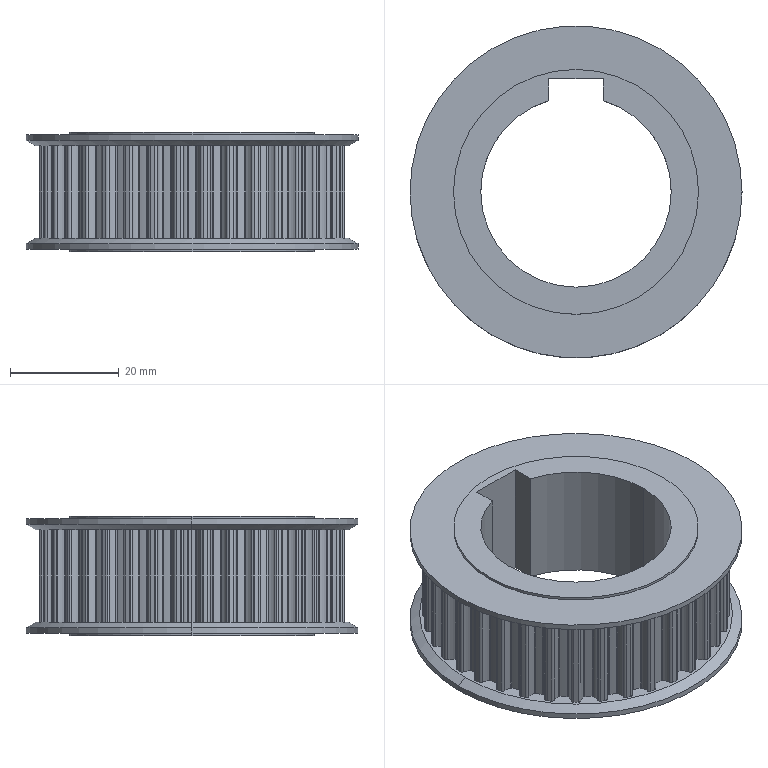Part | STEP file | Y-EAB01-S5M150-36-A-H-d28 tube-turning pulley SGN-2-05 | 1 solid | 345 faces | box 61 x 61 x 22 mm | volume 30514 mm3 | cylinder 332 | plane 9 | cone 4 | commonest cylinder face diameters 1 x88 0.5 x82 6.55 x78 52.8 x37 56.34 x36 45 x4